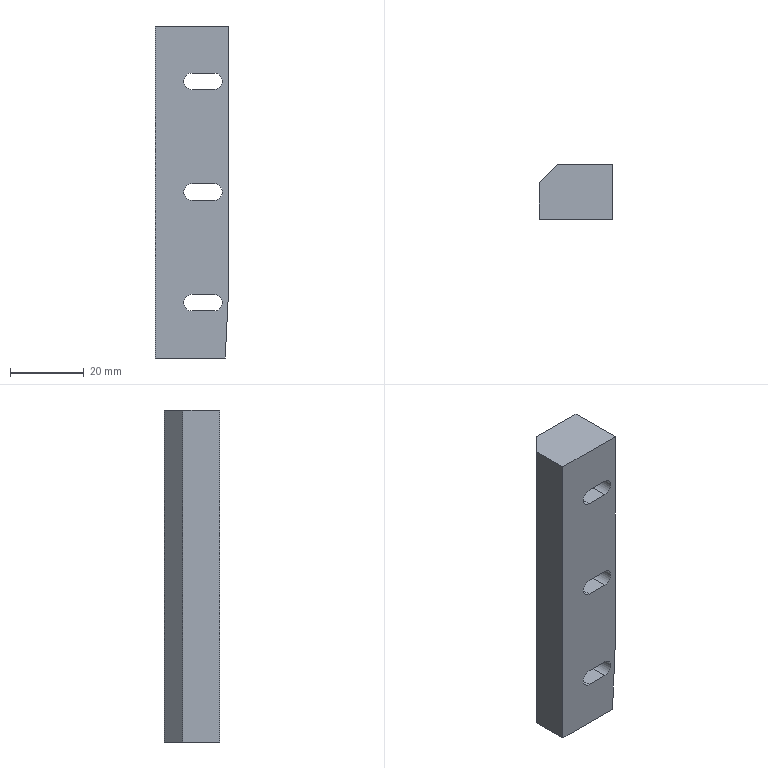Part | SolidWorks | features Cut 3, Chamfer 1, Extrusion 1, LPattern 1 | 1 solid | 36 faces | box 20 x 15 x 90 mm | volume 22961 mm3 | plane 23 | cylinder 13 | commonest cylinder face diameters 7.5 x7 4.5 x6
STEP:
#1=CARTESIAN_POINT('',(0.,9.,32.25));
#2=VERTEX_POINT('',#1);
#3=CARTESIAN_POINT('',(0.,9.,27.75));
#4=VERTEX_POINT('',#3);
#5=CARTESIAN_POINT('',(0.,9.,30.));
#6=DIRECTION('',(0.,-1.,0.));
#7=DIRECTION('',(0.,0.,1.));
#8=AXIS2_PLACEMENT_3D('',#5,#6,#7);
#9=CIRCLE('',#8,2.25);
#10=EDGE_CURVE('',#2,#4,#9,.T.);
#11=ORIENTED_EDGE('',*,*,#10,.F.);
#12=CARTESIAN_POINT('',(0.,0.,32.25));
#13=VERTEX_POINT('',#12);
#14=CARTESIAN_POINT('',(0.,0.,32.25));
#15=DIRECTION('',(0.,1.,0.));
#16=VECTOR('',#15,1000.);
#17=LINE('',#14,#16);
#18=EDGE_CURVE('',#13,#2,#17,.T.);
#19=ORIENTED_EDGE('',*,*,#18,.F.);
#20=CARTESIAN_POINT('',(0.,0.,27.75));
#21=VERTEX_POINT('',#20);
#22=CARTESIAN_POINT('',(0.,0.,30.));
#23=DIRECTION('',(0.,1.,0.));
#24=DIRECTION('',(0.,0.,1.));
#25=AXIS2_PLACEMENT_3D('',#22,#23,#24);
#26=CIRCLE('',#25,2.25);
#27=EDGE_CURVE('',#21,#13,#26,.T.);
#28=ORIENTED_EDGE('',*,*,#27,.F.);
#29=CARTESIAN_POINT('',(0.,0.,27.75));
#30=DIRECTION('',(0.,1.,0.));
#31=VECTOR('',#30,1000.);
#32=LINE('',#29,#31);
#33=EDGE_CURVE('',#21,#4,#32,.T.);
#34=ORIENTED_EDGE('',*,*,#33,.T.);
#35=EDGE_LOOP('',(#11,#19,#28,#34));
#36=FACE_OUTER_BOUND('',#35,.T.);
#37=CARTESIAN_POINT('',(0.,0.,30.));
#38=DIRECTION('',(0.,1.,0.));
#39=DIRECTION('',(0.,0.,1.));
#40=AXIS2_PLACEMENT_3D('',#37,#38,#39);
#41=CYLINDRICAL_SURFACE('',#40,2.25);
#42=ADVANCED_FACE('',(#36),#41,.F.);
#43=CARTESIAN_POINT('',(6.,9.,27.75));
#44=VERTEX_POINT('',#43);
#45=CARTESIAN_POINT('',(0.,9.,27.75));
#46=DIRECTION('',(1.,0.,0.));
#47=VECTOR('',#46,1000.);
#48=LINE('',#45,#47);
#49=EDGE_CURVE('',#4,#44,#48,.T.);
#50=ORIENTED_EDGE('',*,*,#49,.F.);
#51=ORIENTED_EDGE('',*,*,#33,.F.);
#52=CARTESIAN_POINT('',(6.,0.,27.75));
#53=VERTEX_POINT('',#52);
#54=CARTESIAN_POINT('',(0.,0.,27.75));
#55=DIRECTION('',(-1.,0.,0.));
#56=VECTOR('',#55,1000.);
#57=LINE('',#54,#56);
#58=EDGE_CURVE('',#53,#21,#57,.T.);
#59=ORIENTED_EDGE('',*,*,#58,.F.);
#60=CARTESIAN_POINT('',(6.,0.,27.75));
#61=DIRECTION('',(0.,1.,0.));
#62=VECTOR('',#61,1000.);
#63=LINE('',#60,#62);
#64=EDGE_CURVE('',#53,#44,#63,.T.);
#65=ORIENTED_EDGE('',*,*,#64,.T.);
#66=EDGE_LOOP('',(#50,#51,#59,#65));
#67=FACE_OUTER_BOUND('',#66,.T.);
#68=CARTESIAN_POINT('',(0.,0.,27.75));
#69=DIRECTION('',(0.,0.,-1.));
#70=DIRECTION('',(-1.,0.,0.));
#71=AXIS2_PLACEMENT_3D('',#68,#69,#70);
#72=PLANE('',#71);
#73=ADVANCED_FACE('',(#67),#72,.F.);
#74=CARTESIAN_POINT('',(6.,9.,32.25));
#75=VERTEX_POINT('',#74);
#76=CARTESIAN_POINT('',(6.,9.,30.));
#77=DIRECTION('',(0.,-1.,0.));
#78=DIRECTION('',(0.,0.,1.));
#79=AXIS2_PLACEMENT_3D('',#76,#77,#78);
#80=CIRCLE('',#79,2.25);
#81=EDGE_CURVE('',#44,#75,#80,.T.);
#82=ORIENTED_EDGE('',*,*,#81,.F.);
#83=ORIENTED_EDGE('',*,*,#64,.F.);
#84=CARTESIAN_POINT('',(6.,0.,32.25));
#85=VERTEX_POINT('',#84);
#86=CARTESIAN_POINT('',(6.,0.,30.));
#87=DIRECTION('',(0.,1.,0.));
#88=DIRECTION('',(0.,0.,1.));
#89=AXIS2_PLACEMENT_3D('',#86,#87,#88);
#90=CIRCLE('',#89,2.25);
#91=EDGE_CURVE('',#85,#53,#90,.T.);
#92=ORIENTED_EDGE('',*,*,#91,.F.);
#93=CARTESIAN_POINT('',(6.,0.,32.25));
#94=DIRECTION('',(0.,1.,0.));
#95=VECTOR('',#94,1000.);
#96=LINE('',#93,#95);
#97=EDGE_CURVE('',#85,#75,#96,.T.);
#98=ORIENTED_EDGE('',*,*,#97,.T.);
#99=EDGE_LOOP('',(#82,#83,#92,#98));
#100=FACE_OUTER_BOUND('',#99,.T.);
#101=CARTESIAN_POINT('',(6.,0.,30.));
#102=DIRECTION('',(0.,1.,0.));
#103=DIRECTION('',(0.,0.,1.));
#104=AXIS2_PLACEMENT_3D('',#101,#102,#103);
#105=CYLINDRICAL_SURFACE('',#104,2.25);
#106=ADVANCED_FACE('',(#100),#105,.F.);
#107=CARTESIAN_POINT('',(0.,9.,32.25));
#108=DIRECTION('',(-1.,0.,0.));
#109=VECTOR('',#108,1000.);
#110=LINE('',#107,#109);
#111=EDGE_CURVE('',#75,#2,#110,.T.);
#112=ORIENTED_EDGE('',*,*,#111,.F.);
#113=ORIENTED_EDGE('',*,*,#97,.F.);
#114=CARTESIAN_POINT('',(0.,0.,32.25));
#115=DIRECTION('',(1.,0.,0.));
#116=VECTOR('',#115,1000.);
#117=LINE('',#114,#116);
#118=EDGE_CURVE('',#13,#85,#117,.T.);
#119=ORIENTED_EDGE('',*,*,#118,.F.);
#120=ORIENTED_EDGE('',*,*,#18,.T.);
#121=EDGE_LOOP('',(#112,#113,#119,#120));
#122=FACE_OUTER_BOUND('',#121,.T.);
#123=CARTESIAN_POINT('',(0.,0.,32.25));
#124=DIRECTION('',(0.,0.,1.));
#125=DIRECTION('',(1.,0.,0.));
#126=AXIS2_PLACEMENT_3D('',#123,#124,#125);
#127=PLANE('',#126);
#128=ADVANCED_FACE('',(#122),#127,.F.);
#129=CARTESIAN_POINT('',(0.,9.,-27.75));
#130=VERTEX_POINT('',#129);
#131=CARTESIAN_POINT('',(0.,9.,-32.25));
#132=VERTEX_POINT('',#131);
#133=CARTESIAN_POINT('',(0.,9.,-30.));
#134=DIRECTION('',(0.,-1.,0.));
#135=DIRECTION('',(0.,0.,1.));
#136=AXIS2_PLACEMENT_3D('',#133,#134,#135);
#137=CIRCLE('',#136,2.25);
#138=EDGE_CURVE('',#130,#132,#137,.T.);
#139=ORIENTED_EDGE('',*,*,#138,.F.);
#140=CARTESIAN_POINT('',(0.,0.,-27.75));
#141=VERTEX_POINT('',#140);
#142=CARTESIAN_POINT('',(0.,0.,-27.75));
#143=DIRECTION('',(0.,1.,0.));
#144=VECTOR('',#143,1000.);
#145=LINE('',#142,#144);
#146=EDGE_CURVE('',#141,#130,#145,.T.);
#147=ORIENTED_EDGE('',*,*,#146,.F.);
#148=CARTESIAN_POINT('',(0.,0.,-32.25));
#149=VERTEX_POINT('',#148);
#150=CARTESIAN_POINT('',(0.,0.,-30.));
#151=DIRECTION('',(0.,1.,0.));
#152=DIRECTION('',(0.,0.,1.));
#153=AXIS2_PLACEMENT_3D('',#150,#151,#152);
#154=CIRCLE('',#153,2.25);
#155=EDGE_CURVE('',#149,#141,#154,.T.);
#156=ORIENTED_EDGE('',*,*,#155,.F.);
#157=CARTESIAN_POINT('',(0.,0.,-32.25));
#158=DIRECTION('',(0.,1.,0.));
#159=VECTOR('',#158,1000.);
#160=LINE('',#157,#159);
#161=EDGE_CURVE('',#149,#132,#160,.T.);
#162=ORIENTED_EDGE('',*,*,#161,.T.);
#163=EDGE_LOOP('',(#139,#147,#156,#162));
#164=FACE_OUTER_BOUND('',#163,.T.);
#165=CARTESIAN_POINT('',(0.,0.,-30.));
#166=DIRECTION('',(0.,1.,0.));
#167=DIRECTION('',(0.,0.,1.));
#168=AXIS2_PLACEMENT_3D('',#165,#166,#167);
#169=CYLINDRICAL_SURFACE('',#168,2.25);
#170=ADVANCED_FACE('',(#164),#169,.F.);
#171=CARTESIAN_POINT('',(6.,9.,-32.25));
#172=VERTEX_POINT('',#171);
#173=CARTESIAN_POINT('',(0.,9.,-32.25));
#174=DIRECTION('',(1.,0.,0.));
#175=VECTOR('',#174,1000.);
#176=LINE('',#173,#175);
#177=EDGE_CURVE('',#132,#172,#176,.T.);
#178=ORIENTED_EDGE('',*,*,#177,.F.);
#179=ORIENTED_EDGE('',*,*,#161,.F.);
#180=CARTESIAN_POINT('',(6.,0.,-32.25));
#181=VERTEX_POINT('',#180);
#182=CARTESIAN_POINT('',(0.,0.,-32.25));
#183=DIRECTION('',(-1.,0.,0.));
#184=VECTOR('',#183,1000.);
#185=LINE('',#182,#184);
#186=EDGE_CURVE('',#181,#149,#185,.T.);
#187=ORIENTED_EDGE('',*,*,#186,.F.);
#188=CARTESIAN_POINT('',(6.,0.,-32.25));
#189=DIRECTION('',(0.,1.,0.));
#190=VECTOR('',#189,1000.);
#191=LINE('',#188,#190);
#192=EDGE_CURVE('',#181,#172,#191,.T.);
#193=ORIENTED_EDGE('',*,*,#192,.T.);
#194=EDGE_LOOP('',(#178,#179,#187,#193));
#195=FACE_OUTER_BOUND('',#194,.T.);
#196=CARTESIAN_POINT('',(0.,0.,-32.25));
#197=DIRECTION('',(0.,0.,-1.));
#198=DIRECTION('',(-1.,0.,0.));
#199=AXIS2_PLACEMENT_3D('',#196,#197,#198);
#200=PLANE('',#199);
#201=ADVANCED_FACE('',(#195),#200,.F.);
#202=CARTESIAN_POINT('',(6.,9.,-27.75));
#203=VERTEX_POINT('',#202);
#204=CARTESIAN_POINT('',(6.,9.,-30.));
#205=DIRECTION('',(0.,-1.,0.));
#206=DIRECTION('',(0.,0.,1.));
#207=AXIS2_PLACEMENT_3D('',#204,#205,#206);
#208=CIRCLE('',#207,2.25);
#209=EDGE_CURVE('',#172,#203,#208,.T.);
#210=ORIENTED_EDGE('',*,*,#209,.F.);
#211=ORIENTED_EDGE('',*,*,#192,.F.);
#212=CARTESIAN_POINT('',(6.,0.,-27.75));
#213=VERTEX_POINT('',#212);
#214=CARTESIAN_POINT('',(6.,0.,-30.));
#215=DIRECTION('',(0.,1.,0.));
#216=DIRECTION('',(0.,0.,1.));
#217=AXIS2_PLACEMENT_3D('',#214,#215,#216);
#218=CIRCLE('',#217,2.25);
#219=EDGE_CURVE('',#213,#181,#218,.T.);
#220=ORIENTED_EDGE('',*,*,#219,.F.);
#221=CARTESIAN_POINT('',(6.,0.,-27.75));
#222=DIRECTION('',(0.,1.,0.));
#223=VECTOR('',#222,1000.);
#224=LINE('',#221,#223);
#225=EDGE_CURVE('',#213,#203,#224,.T.);
#226=ORIENTED_EDGE('',*,*,#225,.T.);
#227=EDGE_LOOP('',(#210,#211,#220,#226));
#228=FACE_OUTER_BOUND('',#227,.T.);
#229=CARTESIAN_POINT('',(6.,0.,-30.));
#230=DIRECTION('',(0.,1.,0.));
#231=DIRECTION('',(0.,0.,1.));
#232=AXIS2_PLACEMENT_3D('',#229,#230,#231);
#233=CYLINDRICAL_SURFACE('',#232,2.25);
#234=ADVANCED_FACE('',(#228),#233,.F.);
#235=CARTESIAN_POINT('',(0.,9.,-27.75));
#236=DIRECTION('',(-1.,0.,0.));
#237=VECTOR('',#236,1000.);
#238=LINE('',#235,#237);
#239=EDGE_CURVE('',#203,#130,#238,.T.);
#240=ORIENTED_EDGE('',*,*,#239,.F.);
#241=ORIENTED_EDGE('',*,*,#225,.F.);
#242=CARTESIAN_POINT('',(0.,0.,-27.75));
#243=DIRECTION('',(1.,0.,0.));
#244=VECTOR('',#243,1000.);
#245=LINE('',#242,#244);
#246=EDGE_CURVE('',#141,#213,#245,.T.);
#247=ORIENTED_EDGE('',*,*,#246,.F.);
#248=ORIENTED_EDGE('',*,*,#146,.T.);
#249=EDGE_LOOP('',(#240,#241,#247,#248));
#250=FACE_OUTER_BOUND('',#249,.T.);
#251=CARTESIAN_POINT('',(0.,0.,-27.75));
#252=DIRECTION('',(0.,0.,1.));
#253=DIRECTION('',(1.,0.,0.));
#254=AXIS2_PLACEMENT_3D('',#251,#252,#253);
#255=PLANE('',#254);
#256=ADVANCED_FACE('',(#250),#255,.F.);
#257=CARTESIAN_POINT('',(0.,9.,2.25));
#258=VERTEX_POINT('',#257);
#259=CARTESIAN_POINT('',(0.,9.,-2.25));
#260=VERTEX_POINT('',#259);
#261=CARTESIAN_POINT('',(0.,9.,0.));
#262=DIRECTION('',(0.,-1.,0.));
#263=DIRECTION('',(0.,0.,1.));
#264=AXIS2_PLACEMENT_3D('',#261,#262,#263);
#265=CIRCLE('',#264,2.25);
#266=EDGE_CURVE('',#258,#260,#265,.T.);
#267=ORIENTED_EDGE('',*,*,#266,.F.);
#268=CARTESIAN_POINT('',(0.,0.,2.25));
#269=VERTEX_POINT('',#268);
#270=CARTESIAN_POINT('',(0.,0.,2.25));
#271=DIRECTION('',(0.,1.,0.));
#272=VECTOR('',#271,1000.);
#273=LINE('',#270,#272);
#274=EDGE_CURVE('',#269,#258,#273,.T.);
#275=ORIENTED_EDGE('',*,*,#274,.F.);
#276=CARTESIAN_POINT('',(0.,0.,-2.25));
#277=VERTEX_POINT('',#276);
#278=CARTESIAN_POINT('',(0.,0.,0.));
#279=DIRECTION('',(0.,1.,0.));
#280=DIRECTION('',(0.,0.,1.));
#281=AXIS2_PLACEMENT_3D('',#278,#279,#280);
#282=CIRCLE('',#281,2.25);
#283=EDGE_CURVE('',#277,#269,#282,.T.);
#284=ORIENTED_EDGE('',*,*,#283,.F.);
#285=CARTESIAN_POINT('',(0.,0.,-2.25));
#286=DIRECTION('',(0.,1.,0.));
#287=VECTOR('',#286,1000.);
#288=LINE('',#285,#287);
#289=EDGE_CURVE('',#277,#260,#288,.T.);
#290=ORIENTED_EDGE('',*,*,#289,.T.);
#291=EDGE_LOOP('',(#267,#275,#284,#290));
#292=FACE_OUTER_BOUND('',#291,.T.);
#293=CARTESIAN_POINT('',(0.,0.,0.));
#294=DIRECTION('',(0.,1.,0.));
#295=DIRECTION('',(0.,0.,1.));
#296=AXIS2_PLACEMENT_3D('',#293,#294,#295);
#297=CYLINDRICAL_SURFACE('',#296,2.25);
#298=ADVANCED_FACE('',(#292),#297,.F.);
#299=CARTESIAN_POINT('',(6.,9.,-2.25));
#300=VERTEX_POINT('',#299);
#301=CARTESIAN_POINT('',(0.,9.,-2.25));
#302=DIRECTION('',(1.,0.,0.));
#303=VECTOR('',#302,1000.);
#304=LINE('',#301,#303);
#305=EDGE_CURVE('',#260,#300,#304,.T.);
#306=ORIENTED_EDGE('',*,*,#305,.F.);
#307=ORIENTED_EDGE('',*,*,#289,.F.);
#308=CARTESIAN_POINT('',(6.,0.,-2.25));
#309=VERTEX_POINT('',#308);
#310=CARTESIAN_POINT('',(0.,0.,-2.25));
#311=DIRECTION('',(-1.,0.,0.));
#312=VECTOR('',#311,1000.);
#313=LINE('',#310,#312);
#314=EDGE_CURVE('',#309,#277,#313,.T.);
#315=ORIENTED_EDGE('',*,*,#314,.F.);
#316=CARTESIAN_POINT('',(6.,0.,-2.25));
#317=DIRECTION('',(0.,1.,0.));
#318=VECTOR('',#317,1000.);
#319=LINE('',#316,#318);
#320=EDGE_CURVE('',#309,#300,#319,.T.);
#321=ORIENTED_EDGE('',*,*,#320,.T.);
#322=EDGE_LOOP('',(#306,#307,#315,#321));
#323=FACE_OUTER_BOUND('',#322,.T.);
#324=CARTESIAN_POINT('',(0.,0.,-2.25));
#325=DIRECTION('',(0.,0.,-1.));
#326=DIRECTION('',(-1.,0.,0.));
#327=AXIS2_PLACEMENT_3D('',#324,#325,#326);
#328=PLANE('',#327);
#329=ADVANCED_FACE('',(#323),#328,.F.);
#330=CARTESIAN_POINT('',(6.,9.,2.25));
#331=VERTEX_POINT('',#330);
#332=CARTESIAN_POINT('',(6.,9.,0.));
#333=DIRECTION('',(0.,-1.,0.));
#334=DIRECTION('',(0.,0.,1.));
#335=AXIS2_PLACEMENT_3D('',#332,#333,#334);
#336=CIRCLE('',#335,2.25);
#337=EDGE_CURVE('',#300,#331,#336,.T.);
#338=ORIENTED_EDGE('',*,*,#337,.F.);
#339=ORIENTED_EDGE('',*,*,#320,.F.);
#340=CARTESIAN_POINT('',(6.,0.,2.25));
#341=VERTEX_POINT('',#340);
#342=CARTESIAN_POINT('',(6.,0.,0.));
#343=DIRECTION('',(0.,1.,0.));
#344=DIRECTION('',(0.,0.,1.));
#345=AXIS2_PLACEMENT_3D('',#342,#343,#344);
#346=CIRCLE('',#345,2.25);
#347=EDGE_CURVE('',#341,#309,#346,.T.);
#348=ORIENTED_EDGE('',*,*,#347,.F.);
#349=CARTESIAN_POINT('',(6.,0.,2.25));
#350=DIRECTION('',(0.,1.,0.));
#351=VECTOR('',#350,1000.);
#352=LINE('',#349,#351);
#353=EDGE_CURVE('',#341,#331,#352,.T.);
#354=ORIENTED_EDGE('',*,*,#353,.T.);
#355=EDGE_LOOP('',(#338,#339,#348,#354));
#356=FACE_OUTER_BOUND('',#355,.T.);
#357=CARTESIAN_POINT('',(6.,0.,0.));
#358=DIRECTION('',(0.,1.,0.));
#359=DIRECTION('',(0.,0.,1.));
#360=AXIS2_PLACEMENT_3D('',#357,#358,#359);
#361=CYLINDRICAL_SURFACE('',#360,2.25);
#362=ADVANCED_FACE('',(#356),#361,.F.);
#363=CARTESIAN_POINT('',(0.,9.,2.25));
#364=DIRECTION('',(-1.,0.,0.));
#365=VECTOR('',#364,1000.);
#366=LINE('',#363,#365);
#367=EDGE_CURVE('',#331,#258,#366,.T.);
#368=ORIENTED_EDGE('',*,*,#367,.F.);
#369=ORIENTED_EDGE('',*,*,#353,.F.);
#370=CARTESIAN_POINT('',(0.,0.,2.25));
#371=DIRECTION('',(1.,0.,0.));
#372=VECTOR('',#371,1000.);
#373=LINE('',#370,#372);
#374=EDGE_CURVE('',#269,#341,#373,.T.);
#375=ORIENTED_EDGE('',*,*,#374,.F.);
#376=ORIENTED_EDGE('',*,*,#274,.T.);
#377=EDGE_LOOP('',(#368,#369,#375,#376));
#378=FACE_OUTER_BOUND('',#377,.T.);
#379=CARTESIAN_POINT('',(0.,0.,2.25));
#380=DIRECTION('',(0.,0.,1.));
#381=DIRECTION('',(1.,0.,0.));
#382=AXIS2_PLACEMENT_3D('',#379,#380,#381);
#383=PLANE('',#382);
#384=ADVANCED_FACE('',(#378),#383,.F.);
#385=CARTESIAN_POINT('',(10.,0.,45.));
#386=VERTEX_POINT('',#385);
#387=CARTESIAN_POINT('',(10.,0.,-25.));
#388=VERTEX_POINT('',#387);
#389=CARTESIAN_POINT('',(10.,0.,-45.));
#390=DIRECTION('',(0.,0.,-1.));
#391=VECTOR('',#390,1000.);
#392=LINE('',#389,#391);
#393=EDGE_CURVE('',#386,#388,#392,.T.);
#394=ORIENTED_EDGE('',*,*,#393,.T.);
#395=CARTESIAN_POINT('',(10.,15.,-25.));
#396=VERTEX_POINT('',#395);
#397=CARTESIAN_POINT('',(10.,0.,-25.));
#398=DIRECTION('',(0.,1.,0.));
#399=VECTOR('',#398,1000.);
#400=LINE('',#397,#399);
#401=EDGE_CURVE('',#388,#396,#400,.T.);
#402=ORIENTED_EDGE('',*,*,#401,.T.);
#403=CARTESIAN_POINT('',(10.,15.,45.));
#404=VERTEX_POINT('',#403);
#405=CARTESIAN_POINT('',(10.,15.,-45.));
#406=DIRECTION('',(0.,0.,-1.));
#407=VECTOR('',#406,1000.);
#408=LINE('',#405,#407);
#409=EDGE_CURVE('',#404,#396,#408,.T.);
#410=ORIENTED_EDGE('',*,*,#409,.F.);
#411=CARTESIAN_POINT('',(10.,15.,45.));
#412=DIRECTION('',(0.,-1.,0.));
#413=VECTOR('',#412,1000.);
#414=LINE('',#411,#413);
#415=EDGE_CURVE('',#404,#386,#414,.T.);
#416=ORIENTED_EDGE('',*,*,#415,.T.);
#417=EDGE_LOOP('',(#394,#402,#410,#416));
#418=FACE_OUTER_BOUND('',#417,.T.);
#419=CARTESIAN_POINT('',(10.,15.,-45.));
#420=DIRECTION('',(-1.,0.,0.));
#421=DIRECTION('',(0.,0.,1.));
#422=AXIS2_PLACEMENT_3D('',#419,#420,#421);
#423=PLANE('',#422);
#424=ADVANCED_FACE('',(#418),#423,.F.);
#425=CARTESIAN_POINT('',(9.,15.,-45.));
#426=VERTEX_POINT('',#425);
#427=CARTESIAN_POINT('',(-5.,15.,-45.));
#428=VERTEX_POINT('',#427);
#429=CARTESIAN_POINT('',(-10.,15.,-45.));
#430=DIRECTION('',(-1.,0.,0.));
#431=VECTOR('',#430,1000.);
#432=LINE('',#429,#431);
#433=EDGE_CURVE('',#426,#428,#432,.T.);
#434=ORIENTED_EDGE('',*,*,#433,.F.);
#435=CARTESIAN_POINT('',(9.,0.,-45.));
#436=VERTEX_POINT('',#435);
#437=CARTESIAN_POINT('',(9.,0.,-45.));
#438=DIRECTION('',(0.,1.,0.));
#439=VECTOR('',#438,1000.);
#440=LINE('',#437,#439);
#441=EDGE_CURVE('',#436,#426,#440,.T.);
#442=ORIENTED_EDGE('',*,*,#441,.F.);
#443=CARTESIAN_POINT('',(-10.,0.,-45.));
#444=VERTEX_POINT('',#443);
#445=CARTESIAN_POINT('',(-10.,0.,-45.));
#446=DIRECTION('',(-1.,0.,0.));
#447=VECTOR('',#446,1000.);
#448=LINE('',#445,#447);
#449=EDGE_CURVE('',#436,#444,#448,.T.);
#450=ORIENTED_EDGE('',*,*,#449,.T.);
#451=CARTESIAN_POINT('',(-10.,10.,-45.));
#452=VERTEX_POINT('',#451);
#453=CARTESIAN_POINT('',(-10.,15.,-45.));
#454=DIRECTION('',(0.,-1.,0.));
#455=VECTOR('',#454,1000.);
#456=LINE('',#453,#455);
#457=EDGE_CURVE('',#452,#444,#456,.T.);
#458=ORIENTED_EDGE('',*,*,#457,.F.);
#459=CARTESIAN_POINT('',(-5.,15.,-45.));
#460=DIRECTION('',(0.7071,0.7071,0.));
#461=VECTOR('',#460,1000.);
#462=LINE('',#459,#461);
#463=EDGE_CURVE('',#452,#428,#462,.T.);
#464=ORIENTED_EDGE('',*,*,#463,.T.);
#465=EDGE_LOOP('',(#434,#442,#450,#458,#464));
#466=FACE_OUTER_BOUND('',#465,.T.);
#467=CARTESIAN_POINT('',(-10.,15.,-45.));
#468=DIRECTION('',(0.,0.,1.));
#469=DIRECTION('',(1.,0.,0.));
#470=AXIS2_PLACEMENT_3D('',#467,#468,#469);
#471=PLANE('',#470);
#472=ADVANCED_FACE('',(#466),#471,.F.);
#473=CARTESIAN_POINT('',(-10.,10.,45.));
#474=VERTEX_POINT('',#473);
#475=CARTESIAN_POINT('',(-10.,0.,45.));
#476=VERTEX_POINT('',#475);
#477=CARTESIAN_POINT('',(-10.,15.,45.));
#478=DIRECTION('',(0.,-1.,0.));
#479=VECTOR('',#478,1000.);
#480=LINE('',#477,#479);
#481=EDGE_CURVE('',#474,#476,#480,.T.);
#482=ORIENTED_EDGE('',*,*,#481,.F.);
#483=CARTESIAN_POINT('',(-10.,10.,-45.));
#484=DIRECTION('',(0.,0.,-1.));
#485=VECTOR('',#484,1000.);
#486=LINE('',#483,#485);
#487=EDGE_CURVE('',#474,#452,#486,.T.);
#488=ORIENTED_EDGE('',*,*,#487,.T.);
#489=ORIENTED_EDGE('',*,*,#457,.T.);
#490=CARTESIAN_POINT('',(-10.,0.,-45.));
#491=DIRECTION('',(0.,0.,1.));
#492=VECTOR('',#491,1000.);
#493=LINE('',#490,#492);
#494=EDGE_CURVE('',#444,#476,#493,.T.);
#495=ORIENTED_EDGE('',*,*,#494,.T.);
#496=EDGE_LOOP('',(#482,#488,#489,#495));
#497=FACE_OUTER_BOUND('',#496,.T.);
#498=CARTESIAN_POINT('',(-10.,15.,-45.));
#499=DIRECTION('',(1.,0.,0.));
#500=DIRECTION('',(0.,0.,-1.));
#501=AXIS2_PLACEMENT_3D('',#498,#499,#500);
#502=PLANE('',#501);
#503=ADVANCED_FACE('',(#497),#502,.F.);
#504=CARTESIAN_POINT('',(-5.,15.,45.));
#505=VERTEX_POINT('',#504);
#506=CARTESIAN_POINT('',(-10.,15.,45.));
#507=DIRECTION('',(1.,0.,0.));
#508=VECTOR('',#507,1000.);
#509=LINE('',#506,#508);
#510=EDGE_CURVE('',#505,#404,#509,.T.);
#511=ORIENTED_EDGE('',*,*,#510,.F.);
#512=CARTESIAN_POINT('',(-5.,15.,45.));
#513=DIRECTION('',(-0.7071,-0.7071,0.));
#514=VECTOR('',#513,1000.);
#515=LINE('',#512,#514);
#516=EDGE_CURVE('',#505,#474,#515,.T.);
#517=ORIENTED_EDGE('',*,*,#516,.T.);
#518=ORIENTED_EDGE('',*,*,#481,.T.);
#519=CARTESIAN_POINT('',(-10.,0.,45.));
#520=DIRECTION('',(1.,0.,0.));
#521=VECTOR('',#520,1000.);
#522=LINE('',#519,#521);
#523=EDGE_CURVE('',#476,#386,#522,.T.);
#524=ORIENTED_EDGE('',*,*,#523,.T.);
#525=ORIENTED_EDGE('',*,*,#415,.F.);
#526=EDGE_LOOP('',(#511,#517,#518,#524,#525));
#527=FACE_OUTER_BOUND('',#526,.T.);
#528=CARTESIAN_POINT('',(-10.,15.,45.));
#529=DIRECTION('',(0.,0.,-1.));
#530=DIRECTION('',(-1.,0.,0.));
#531=AXIS2_PLACEMENT_3D('',#528,#529,#530);
#532=PLANE('',#531);
#533=ADVANCED_FACE('',(#527),#532,.F.);
#534=CARTESIAN_POINT('',(0.,15.,26.25));
#535=VERTEX_POINT('',#534);
#536=CARTESIAN_POINT('',(0.,15.,33.75));
#537=VERTEX_POINT('',#536);
#538=CARTESIAN_POINT('',(0.,15.,30.));
#539=DIRECTION('',(0.,1.,0.));
#540=DIRECTION('',(0.,0.,1.));
#541=AXIS2_PLACEMENT_3D('',#538,#539,#540);
#542=CIRCLE('',#541,3.75);
#543=EDGE_CURVE('',#535,#537,#542,.T.);
#544=ORIENTED_EDGE('',*,*,#543,.F.);
#545=CARTESIAN_POINT('',(6.,15.,26.25));
#546=VERTEX_POINT('',#545);
#547=CARTESIAN_POINT('',(6.,15.,26.25));
#548=DIRECTION('',(-1.,0.,0.));
#549=VECTOR('',#548,1000.);
#550=LINE('',#547,#549);
#551=EDGE_CURVE('',#546,#535,#550,.T.);
#552=ORIENTED_EDGE('',*,*,#551,.F.);
#553=CARTESIAN_POINT('',(6.,15.,33.75));
#554=VERTEX_POINT('',#553);
#555=CARTESIAN_POINT('',(6.,15.,30.));
#556=DIRECTION('',(0.,1.,0.));
#557=DIRECTION('',(0.,0.,1.));
#558=AXIS2_PLACEMENT_3D('',#555,#556,#557);
#559=CIRCLE('',#558,3.75);
#560=EDGE_CURVE('',#554,#546,#559,.T.);
#561=ORIENTED_EDGE('',*,*,#560,.F.);
#562=CARTESIAN_POINT('',(0.,15.,33.75));
#563=DIRECTION('',(1.,0.,0.));
#564=VECTOR('',#563,1000.);
#565=LINE('',#562,#564);
#566=EDGE_CURVE('',#537,#554,#565,.T.);
#567=ORIENTED_EDGE('',*,*,#566,.F.);
#568=EDGE_LOOP('',(#544,#552,#561,#567));
#569=FACE_BOUND('',#568,.T.);
#570=CARTESIAN_POINT('',(9.731,15.,-30.374));
#571=VERTEX_POINT('',#570);
#572=CARTESIAN_POINT('',(6.,15.,-33.75));
#573=VERTEX_POINT('',#572);
#574=CARTESIAN_POINT('',(6.,15.,-30.));
#575=DIRECTION('',(0.,1.,0.));
#576=DIRECTION('',(0.,0.,1.));
#577=AXIS2_PLACEMENT_3D('',#574,#575,#576);
#578=CIRCLE('',#577,3.75);
#579=EDGE_CURVE('',#571,#573,#578,.T.);
#580=ORIENTED_EDGE('',*,*,#579,.F.);
#581=CARTESIAN_POINT('',(10.,15.,-25.));
#582=DIRECTION('',(0.04994,0.,0.9988));
#583=VECTOR('',#582,1000.);
#584=LINE('',#581,#583);
#585=EDGE_CURVE('',#426,#571,#584,.T.);
#586=ORIENTED_EDGE('',*,*,#585,.F.);
#587=ORIENTED_EDGE('',*,*,#433,.T.);
#588=CARTESIAN_POINT('',(-5.,15.,45.));
#589=DIRECTION('',(0.,0.,1.));
#590=VECTOR('',#589,1000.);
#591=LINE('',#588,#590);
#592=EDGE_CURVE('',#428,#505,#591,.T.);
#593=ORIENTED_EDGE('',*,*,#592,.T.);
#594=ORIENTED_EDGE('',*,*,#510,.T.);
#595=ORIENTED_EDGE('',*,*,#409,.T.);
#596=CARTESIAN_POINT('',(9.75,15.,-30.));
#597=VERTEX_POINT('',#596);
#598=CARTESIAN_POINT('',(10.,15.,-25.));
#599=DIRECTION('',(0.04994,0.,0.9988));
#600=VECTOR('',#599,1000.);
#601=LINE('',#598,#600);
#602=EDGE_CURVE('',#597,#396,#601,.T.);
#603=ORIENTED_EDGE('',*,*,#602,.F.);
#604=CARTESIAN_POINT('',(6.,15.,-26.25));
#605=VERTEX_POINT('',#604);
#606=CARTESIAN_POINT('',(6.,15.,-30.));
#607=DIRECTION('',(0.,1.,0.));
#608=DIRECTION('',(0.,0.,1.));
#609=AXIS2_PLACEMENT_3D('',#606,#607,#608);
#610=CIRCLE('',#609,3.75);
#611=EDGE_CURVE('',#605,#597,#610,.T.);
#612=ORIENTED_EDGE('',*,*,#611,.F.);
#613=CARTESIAN_POINT('',(0.,15.,-26.25));
#614=VERTEX_POINT('',#613);
#615=CARTESIAN_POINT('',(0.,15.,-26.25));
#616=DIRECTION('',(1.,0.,0.));
#617=VECTOR('',#616,1000.);
#618=LINE('',#615,#617);
#619=EDGE_CURVE('',#614,#605,#618,.T.);
#620=ORIENTED_EDGE('',*,*,#619,.F.);
#621=CARTESIAN_POINT('',(0.,15.,-33.75));
#622=VERTEX_POINT('',#621);
#623=CARTESIAN_POINT('',(0.,15.,-30.));
#624=DIRECTION('',(0.,1.,0.));
#625=DIRECTION('',(0.,0.,1.));
#626=AXIS2_PLACEMENT_3D('',#623,#624,#625);
#627=CIRCLE('',#626,3.75);
#628=EDGE_CURVE('',#622,#614,#627,.T.);
#629=ORIENTED_EDGE('',*,*,#628,.F.);
#630=CARTESIAN_POINT('',(6.,15.,-33.75));
#631=DIRECTION('',(-1.,0.,0.));
#632=VECTOR('',#631,1000.);
#633=LINE('',#630,#632);
#634=EDGE_CURVE('',#573,#622,#633,.T.);
#635=ORIENTED_EDGE('',*,*,#634,.F.);
#636=EDGE_LOOP('',(#580,#586,#587,#593,#594,#595,#603,#612,#620,#629,#635));
#637=FACE_OUTER_BOUND('',#636,.T.);
#638=CARTESIAN_POINT('',(0.,15.,-3.75));
#639=VERTEX_POINT('',#638);
#640=CARTESIAN_POINT('',(0.,15.,3.75));
#641=VERTEX_POINT('',#640);
#642=CARTESIAN_POINT('',(0.,15.,0.));
#643=DIRECTION('',(0.,1.,0.));
#644=DIRECTION('',(0.,0.,1.));
#645=AXIS2_PLACEMENT_3D('',#642,#643,#644);
#646=CIRCLE('',#645,3.75);
#647=EDGE_CURVE('',#639,#641,#646,.T.);
#648=ORIENTED_EDGE('',*,*,#647,.F.);
#649=CARTESIAN_POINT('',(6.,15.,-3.75));
#650=VERTEX_POINT('',#649);
#651=CARTESIAN_POINT('',(6.,15.,-3.75));
#652=DIRECTION('',(-1.,0.,0.));
#653=VECTOR('',#652,1000.);
#654=LINE('',#651,#653);
#655=EDGE_CURVE('',#650,#639,#654,.T.);
#656=ORIENTED_EDGE('',*,*,#655,.F.);
#657=CARTESIAN_POINT('',(6.,15.,3.75));
#658=VERTEX_POINT('',#657);
#659=CARTESIAN_POINT('',(6.,15.,0.));
#660=DIRECTION('',(0.,1.,0.));
#661=DIRECTION('',(0.,0.,1.));
#662=AXIS2_PLACEMENT_3D('',#659,#660,#661);
#663=CIRCLE('',#662,3.75);
#664=EDGE_CURVE('',#658,#650,#663,.T.);
#665=ORIENTED_EDGE('',*,*,#664,.F.);
#666=CARTESIAN_POINT('',(0.,15.,3.75));
#667=DIRECTION('',(1.,0.,0.));
#668=VECTOR('',#667,1000.);
#669=LINE('',#666,#668);
#670=EDGE_CURVE('',#641,#658,#669,.T.);
#671=ORIENTED_EDGE('',*,*,#670,.F.);
#672=EDGE_LOOP('',(#648,#656,#665,#671));
#673=FACE_BOUND('',#672,.T.);
#674=CARTESIAN_POINT('',(0.,15.,0.));
#675=DIRECTION('',(0.,1.,0.));
#676=DIRECTION('',(0.,0.,1.));
#677=AXIS2_PLACEMENT_3D('',#674,#675,#676);
#678=PLANE('',#677);
#679=ADVANCED_FACE('',(#569,#637,#673),#678,.T.);
#680=ORIENTED_EDGE('',*,*,#58,.T.);
#681=ORIENTED_EDGE('',*,*,#27,.T.);
#682=ORIENTED_EDGE('',*,*,#118,.T.);
#683=ORIENTED_EDGE('',*,*,#91,.T.);
#684=EDGE_LOOP('',(#680,#681,#682,#683));
#685=FACE_BOUND('',#684,.T.);
#686=ORIENTED_EDGE('',*,*,#186,.T.);
#687=ORIENTED_EDGE('',*,*,#155,.T.);
#688=ORIENTED_EDGE('',*,*,#246,.T.);
#689=ORIENTED_EDGE('',*,*,#219,.T.);
#690=EDGE_LOOP('',(#686,#687,#688,#689));
#691=FACE_BOUND('',#690,.T.);
#692=ORIENTED_EDGE('',*,*,#314,.T.);
#693=ORIENTED_EDGE('',*,*,#283,.T.);
#694=ORIENTED_EDGE('',*,*,#374,.T.);
#695=ORIENTED_EDGE('',*,*,#347,.T.);
#696=EDGE_LOOP('',(#692,#693,#694,#695));
#697=FACE_BOUND('',#696,.T.);
#698=ORIENTED_EDGE('',*,*,#449,.F.);
#699=CARTESIAN_POINT('',(10.,0.,-25.));
#700=DIRECTION('',(0.04994,0.,0.9988));
#701=VECTOR('',#700,1000.);
#702=LINE('',#699,#701);
#703=EDGE_CURVE('',#436,#388,#702,.T.);
#704=ORIENTED_EDGE('',*,*,#703,.T.);
#705=ORIENTED_EDGE('',*,*,#393,.F.);
#706=ORIENTED_EDGE('',*,*,#523,.F.);
#707=ORIENTED_EDGE('',*,*,#494,.F.);
#708=EDGE_LOOP('',(#698,#704,#705,#706,#707));
#709=FACE_OUTER_BOUND('',#708,.T.);
#710=CARTESIAN_POINT('',(0.,0.,0.));
#711=DIRECTION('',(0.,1.,0.));
#712=DIRECTION('',(0.,0.,1.));
#713=AXIS2_PLACEMENT_3D('',#710,#711,#712);
#714=PLANE('',#713);
#715=ADVANCED_FACE('',(#685,#691,#697,#709),#714,.F.);
#716=ORIENTED_EDGE('',*,*,#463,.F.);
#717=ORIENTED_EDGE('',*,*,#487,.F.);
#718=ORIENTED_EDGE('',*,*,#516,.F.);
#719=ORIENTED_EDGE('',*,*,#592,.F.);
#720=EDGE_LOOP('',(#716,#717,#718,#719));
#721=FACE_OUTER_BOUND('',#720,.T.);
#722=CARTESIAN_POINT('',(-5.,15.,0.));
#723=DIRECTION('',(-0.7071,0.7071,0.));
#724=DIRECTION('',(0.,0.,-1.));
#725=AXIS2_PLACEMENT_3D('',#722,#723,#724);
#726=PLANE('',#725);
#727=ADVANCED_FACE('',(#721),#726,.T.);
#728=CARTESIAN_POINT('',(9.75,9.,-30.));
#729=VERTEX_POINT('',#728);
#730=CARTESIAN_POINT('',(9.731,9.,-30.374));
#731=VERTEX_POINT('',#730);
#732=CARTESIAN_POINT('',(9.75,9.,-30.));
#733=DIRECTION('',(-0.04994,0.,-0.9988));
#734=VECTOR('',#733,1000.);
#735=LINE('',#732,#734);
#736=EDGE_CURVE('',#729,#731,#735,.T.);
#737=ORIENTED_EDGE('',*,*,#736,.F.);
#738=CARTESIAN_POINT('',(9.75,9.,-30.));
#739=DIRECTION('',(0.,1.,0.));
#740=VECTOR('',#739,1000.);
#741=LINE('',#738,#740);
#742=EDGE_CURVE('',#729,#597,#741,.T.);
#743=ORIENTED_EDGE('',*,*,#742,.T.);
#744=ORIENTED_EDGE('',*,*,#602,.T.);
#745=ORIENTED_EDGE('',*,*,#401,.F.);
#746=ORIENTED_EDGE('',*,*,#703,.F.);
#747=ORIENTED_EDGE('',*,*,#441,.T.);
#748=ORIENTED_EDGE('',*,*,#585,.T.);
#749=CARTESIAN_POINT('',(9.731,9.,-30.374));
#750=DIRECTION('',(0.,-1.,0.));
#751=VECTOR('',#750,1000.);
#752=LINE('',#749,#751);
#753=EDGE_CURVE('',#571,#731,#752,.T.);
#754=ORIENTED_EDGE('',*,*,#753,.T.);
#755=EDGE_LOOP('',(#737,#743,#744,#745,#746,#747,#748,#754));
#756=FACE_OUTER_BOUND('',#755,.T.);
#757=CARTESIAN_POINT('',(10.,0.,-25.));
#758=DIRECTION('',(-0.9988,0.,0.04994));
#759=DIRECTION('',(0.04994,0.,0.9988));
#760=AXIS2_PLACEMENT_3D('',#757,#758,#759);
#761=PLANE('',#760);
#762=ADVANCED_FACE('',(#756),#761,.F.);
#763=CARTESIAN_POINT('',(0.,9.,-3.75));
#764=VERTEX_POINT('',#763);
#765=CARTESIAN_POINT('',(0.,9.,3.75));
#766=VERTEX_POINT('',#765);
#767=CARTESIAN_POINT('',(0.,9.,0.));
#768=DIRECTION('',(0.,1.,0.));
#769=DIRECTION('',(0.,0.,1.));
#770=AXIS2_PLACEMENT_3D('',#767,#768,#769);
#771=CIRCLE('',#770,3.75);
#772=EDGE_CURVE('',#764,#766,#771,.T.);
#773=ORIENTED_EDGE('',*,*,#772,.T.);
#774=CARTESIAN_POINT('',(6.,9.,3.75));
#775=VERTEX_POINT('',#774);
#776=CARTESIAN_POINT('',(0.,9.,3.75));
#777=DIRECTION('',(1.,0.,0.));
#778=VECTOR('',#777,1000.);
#779=LINE('',#776,#778);
#780=EDGE_CURVE('',#766,#775,#779,.T.);
#781=ORIENTED_EDGE('',*,*,#780,.T.);
#782=CARTESIAN_POINT('',(6.,9.,-3.75));
#783=VERTEX_POINT('',#782);
#784=CARTESIAN_POINT('',(6.,9.,0.));
#785=DIRECTION('',(0.,1.,0.));
#786=DIRECTION('',(0.,0.,1.));
#787=AXIS2_PLACEMENT_3D('',#784,#785,#786);
#788=CIRCLE('',#787,3.75);
#789=EDGE_CURVE('',#775,#783,#788,.T.);
#790=ORIENTED_EDGE('',*,*,#789,.T.);
#791=CARTESIAN_POINT('',(6.,9.,-3.75));
#792=DIRECTION('',(-1.,0.,0.));
#793=VECTOR('',#792,1000.);
#794=LINE('',#791,#793);
#795=EDGE_CURVE('',#783,#764,#794,.T.);
#796=ORIENTED_EDGE('',*,*,#795,.T.);
#797=EDGE_LOOP('',(#773,#781,#790,#796));
#798=FACE_OUTER_BOUND('',#797,.T.);
#799=ORIENTED_EDGE('',*,*,#266,.T.);
#800=ORIENTED_EDGE('',*,*,#305,.T.);
#801=ORIENTED_EDGE('',*,*,#337,.T.);
#802=ORIENTED_EDGE('',*,*,#367,.T.);
#803=EDGE_LOOP('',(#799,#800,#801,#802));
#804=FACE_BOUND('',#803,.T.);
#805=CARTESIAN_POINT('',(0.,9.,0.));
#806=DIRECTION('',(0.,1.,0.));
#807=DIRECTION('',(0.,0.,1.));
#808=AXIS2_PLACEMENT_3D('',#805,#806,#807);
#809=PLANE('',#808);
#810=ADVANCED_FACE('',(#798,#804),#809,.T.);
#811=ORIENTED_EDGE('',*,*,#647,.T.);
#812=CARTESIAN_POINT('',(0.,9.,3.75));
#813=DIRECTION('',(0.,1.,0.));
#814=VECTOR('',#813,1000.);
#815=LINE('',#812,#814);
#816=EDGE_CURVE('',#766,#641,#815,.T.);
#817=ORIENTED_EDGE('',*,*,#816,.F.);
#818=ORIENTED_EDGE('',*,*,#772,.F.);
#819=CARTESIAN_POINT('',(0.,9.,-3.75));
#820=DIRECTION('',(0.,1.,0.));
#821=VECTOR('',#820,1000.);
#822=LINE('',#819,#821);
#823=EDGE_CURVE('',#764,#639,#822,.T.);
#824=ORIENTED_EDGE('',*,*,#823,.T.);
#825=EDGE_LOOP('',(#811,#817,#818,#824));
#826=FACE_OUTER_BOUND('',#825,.T.);
#827=CARTESIAN_POINT('',(0.,9.,0.));
#828=DIRECTION('',(0.,1.,0.));
#829=DIRECTION('',(0.,0.,1.));
#830=AXIS2_PLACEMENT_3D('',#827,#828,#829);
#831=CYLINDRICAL_SURFACE('',#830,3.75);
#832=ADVANCED_FACE('',(#826),#831,.F.);
#833=ORIENTED_EDGE('',*,*,#655,.T.);
#834=ORIENTED_EDGE('',*,*,#823,.F.);
#835=ORIENTED_EDGE('',*,*,#795,.F.);
#836=CARTESIAN_POINT('',(6.,9.,-3.75));
#837=DIRECTION('',(0.,1.,0.));
#838=VECTOR('',#837,1000.);
#839=LINE('',#836,#838);
#840=EDGE_CURVE('',#783,#650,#839,.T.);
#841=ORIENTED_EDGE('',*,*,#840,.T.);
#842=EDGE_LOOP('',(#833,#834,#835,#841));
#843=FACE_OUTER_BOUND('',#842,.T.);
#844=CARTESIAN_POINT('',(6.,9.,-3.75));
#845=DIRECTION('',(0.,0.,-1.));
#846=DIRECTION('',(-1.,0.,0.));
#847=AXIS2_PLACEMENT_3D('',#844,#845,#846);
#848=PLANE('',#847);
#849=ADVANCED_FACE('',(#843),#848,.F.);
#850=ORIENTED_EDGE('',*,*,#664,.T.);
#851=ORIENTED_EDGE('',*,*,#840,.F.);
#852=ORIENTED_EDGE('',*,*,#789,.F.);
#853=CARTESIAN_POINT('',(6.,9.,3.75));
#854=DIRECTION('',(0.,1.,0.));
#855=VECTOR('',#854,1000.);
#856=LINE('',#853,#855);
#857=EDGE_CURVE('',#775,#658,#856,.T.);
#858=ORIENTED_EDGE('',*,*,#857,.T.);
#859=EDGE_LOOP('',(#850,#851,#852,#858));
#860=FACE_OUTER_BOUND('',#859,.T.);
#861=CARTESIAN_POINT('',(6.,9.,0.));
#862=DIRECTION('',(0.,1.,0.));
#863=DIRECTION('',(0.,0.,1.));
#864=AXIS2_PLACEMENT_3D('',#861,#862,#863);
#865=CYLINDRICAL_SURFACE('',#864,3.75);
#866=ADVANCED_FACE('',(#860),#865,.F.);
#867=ORIENTED_EDGE('',*,*,#670,.T.);
#868=ORIENTED_EDGE('',*,*,#857,.F.);
#869=ORIENTED_EDGE('',*,*,#780,.F.);
#870=ORIENTED_EDGE('',*,*,#816,.T.);
#871=EDGE_LOOP('',(#867,#868,#869,#870));
#872=FACE_OUTER_BOUND('',#871,.T.);
#873=CARTESIAN_POINT('',(0.,9.,3.75));
#874=DIRECTION('',(0.,0.,1.));
#875=DIRECTION('',(1.,0.,0.));
#876=AXIS2_PLACEMENT_3D('',#873,#874,#875);
#877=PLANE('',#876);
#878=ADVANCED_FACE('',(#872),#877,.F.);
#879=CARTESIAN_POINT('',(6.,9.,-26.25));
#880=VERTEX_POINT('',#879);
#881=CARTESIAN_POINT('',(6.,9.,-30.));
#882=DIRECTION('',(0.,1.,0.));
#883=DIRECTION('',(0.,0.,1.));
#884=AXIS2_PLACEMENT_3D('',#881,#882,#883);
#885=CIRCLE('',#884,3.75);
#886=EDGE_CURVE('',#880,#729,#885,.T.);
#887=ORIENTED_EDGE('',*,*,#886,.F.);
#888=CARTESIAN_POINT('',(6.,9.,-26.25));
#889=DIRECTION('',(0.,1.,0.));
#890=VECTOR('',#889,1000.);
#891=LINE('',#888,#890);
#892=EDGE_CURVE('',#880,#605,#891,.T.);
#893=ORIENTED_EDGE('',*,*,#892,.T.);
#894=ORIENTED_EDGE('',*,*,#611,.T.);
#895=ORIENTED_EDGE('',*,*,#742,.F.);
#896=EDGE_LOOP('',(#887,#893,#894,#895));
#897=FACE_OUTER_BOUND('',#896,.T.);
#898=CARTESIAN_POINT('',(6.,9.,-30.));
#899=DIRECTION('',(0.,1.,0.));
#900=DIRECTION('',(0.,0.,1.));
#901=AXIS2_PLACEMENT_3D('',#898,#899,#900);
#902=CYLINDRICAL_SURFACE('',#901,3.75);
#903=ADVANCED_FACE('',(#897),#902,.F.);
#904=ORIENTED_EDGE('',*,*,#579,.T.);
#905=CARTESIAN_POINT('',(6.,9.,-33.75));
#906=VERTEX_POINT('',#905);
#907=CARTESIAN_POINT('',(6.,9.,-33.75));
#908=DIRECTION('',(0.,1.,0.));
#909=VECTOR('',#908,1000.);
#910=LINE('',#907,#909);
#911=EDGE_CURVE('',#906,#573,#910,.T.);
#912=ORIENTED_EDGE('',*,*,#911,.F.);
#913=CARTESIAN_POINT('',(6.,9.,-30.));
#914=DIRECTION('',(0.,1.,0.));
#915=DIRECTION('',(0.,0.,1.));
#916=AXIS2_PLACEMENT_3D('',#913,#914,#915);
#917=CIRCLE('',#916,3.75);
#918=EDGE_CURVE('',#731,#906,#917,.T.);
#919=ORIENTED_EDGE('',*,*,#918,.F.);
#920=ORIENTED_EDGE('',*,*,#753,.F.);
#921=EDGE_LOOP('',(#904,#912,#919,#920));
#922=FACE_OUTER_BOUND('',#921,.T.);
#923=CARTESIAN_POINT('',(6.,9.,-30.));
#924=DIRECTION('',(0.,1.,0.));
#925=DIRECTION('',(0.,0.,1.));
#926=AXIS2_PLACEMENT_3D('',#923,#924,#925);
#927=CYLINDRICAL_SURFACE('',#926,3.75);
#928=ADVANCED_FACE('',(#922),#927,.F.);
#929=ORIENTED_EDGE('',*,*,#138,.T.);
#930=ORIENTED_EDGE('',*,*,#177,.T.);
#931=ORIENTED_EDGE('',*,*,#209,.T.);
#932=ORIENTED_EDGE('',*,*,#239,.T.);
#933=EDGE_LOOP('',(#929,#930,#931,#932));
#934=FACE_BOUND('',#933,.T.);
#935=ORIENTED_EDGE('',*,*,#736,.T.);
#936=ORIENTED_EDGE('',*,*,#918,.T.);
#937=CARTESIAN_POINT('',(0.,9.,-33.75));
#938=VERTEX_POINT('',#937);
#939=CARTESIAN_POINT('',(6.,9.,-33.75));
#940=DIRECTION('',(-1.,0.,0.));
#941=VECTOR('',#940,1000.);
#942=LINE('',#939,#941);
#943=EDGE_CURVE('',#906,#938,#942,.T.);
#944=ORIENTED_EDGE('',*,*,#943,.T.);
#945=CARTESIAN_POINT('',(0.,9.,-26.25));
#946=VERTEX_POINT('',#945);
#947=CARTESIAN_POINT('',(0.,9.,-30.));
#948=DIRECTION('',(0.,1.,0.));
#949=DIRECTION('',(0.,0.,1.));
#950=AXIS2_PLACEMENT_3D('',#947,#948,#949);
#951=CIRCLE('',#950,3.75);
#952=EDGE_CURVE('',#938,#946,#951,.T.);
#953=ORIENTED_EDGE('',*,*,#952,.T.);
#954=CARTESIAN_POINT('',(0.,9.,-26.25));
#955=DIRECTION('',(1.,0.,0.));
#956=VECTOR('',#955,1000.);
#957=LINE('',#954,#956);
#958=EDGE_CURVE('',#946,#880,#957,.T.);
#959=ORIENTED_EDGE('',*,*,#958,.T.);
#960=ORIENTED_EDGE('',*,*,#886,.T.);
#961=EDGE_LOOP('',(#935,#936,#944,#953,#959,#960));
#962=FACE_OUTER_BOUND('',#961,.T.);
#963=CARTESIAN_POINT('',(0.,9.,-30.));
#964=DIRECTION('',(0.,1.,0.));
#965=DIRECTION('',(0.,0.,1.));
#966=AXIS2_PLACEMENT_3D('',#963,#964,#965);
#967=PLANE('',#966);
#968=ADVANCED_FACE('',(#934,#962),#967,.T.);
#969=ORIENTED_EDGE('',*,*,#628,.T.);
#970=CARTESIAN_POINT('',(0.,9.,-26.25));
#971=DIRECTION('',(0.,1.,0.));
#972=VECTOR('',#971,1000.);
#973=LINE('',#970,#972);
#974=EDGE_CURVE('',#946,#614,#973,.T.);
#975=ORIENTED_EDGE('',*,*,#974,.F.);
#976=ORIENTED_EDGE('',*,*,#952,.F.);
#977=CARTESIAN_POINT('',(0.,9.,-33.75));
#978=DIRECTION('',(0.,1.,0.));
#979=VECTOR('',#978,1000.);
#980=LINE('',#977,#979);
#981=EDGE_CURVE('',#938,#622,#980,.T.);
#982=ORIENTED_EDGE('',*,*,#981,.T.);
#983=EDGE_LOOP('',(#969,#975,#976,#982));
#984=FACE_OUTER_BOUND('',#983,.T.);
#985=CARTESIAN_POINT('',(0.,9.,-30.));
#986=DIRECTION('',(0.,1.,0.));
#987=DIRECTION('',(0.,0.,1.));
#988=AXIS2_PLACEMENT_3D('',#985,#986,#987);
#989=CYLINDRICAL_SURFACE('',#988,3.75);
#990=ADVANCED_FACE('',(#984),#989,.F.);
#991=ORIENTED_EDGE('',*,*,#634,.T.);
#992=ORIENTED_EDGE('',*,*,#981,.F.);
#993=ORIENTED_EDGE('',*,*,#943,.F.);
#994=ORIENTED_EDGE('',*,*,#911,.T.);
#995=EDGE_LOOP('',(#991,#992,#993,#994));
#996=FACE_OUTER_BOUND('',#995,.T.);
#997=CARTESIAN_POINT('',(6.,9.,-33.75));
#998=DIRECTION('',(0.,0.,-1.));
#999=DIRECTION('',(-1.,0.,0.));
#1000=AXIS2_PLACEMENT_3D('',#997,#998,#999);
#1001=PLANE('',#1000);
#1002=ADVANCED_FACE('',(#996),#1001,.F.);
#1003=ORIENTED_EDGE('',*,*,#619,.T.);
#1004=ORIENTED_EDGE('',*,*,#892,.F.);
#1005=ORIENTED_EDGE('',*,*,#958,.F.);
#1006=ORIENTED_EDGE('',*,*,#974,.T.);
#1007=EDGE_LOOP('',(#1003,#1004,#1005,#1006));
#1008=FACE_OUTER_BOUND('',#1007,.T.);
#1009=CARTESIAN_POINT('',(0.,9.,-26.25));
#1010=DIRECTION('',(0.,0.,1.));
#1011=DIRECTION('',(1.,0.,0.));
#1012=AXIS2_PLACEMENT_3D('',#1009,#1010,#1011);
#1013=PLANE('',#1012);
#1014=ADVANCED_FACE('',(#1008),#1013,.F.);
#1015=CARTESIAN_POINT('',(0.,9.,26.25));
#1016=VERTEX_POINT('',#1015);
#1017=CARTESIAN_POINT('',(0.,9.,33.75));
#1018=VERTEX_POINT('',#1017);
#1019=CARTESIAN_POINT('',(0.,9.,30.));
#1020=DIRECTION('',(0.,1.,0.));
#1021=DIRECTION('',(0.,0.,1.));
#1022=AXIS2_PLACEMENT_3D('',#1019,#1020,#1021);
#1023=CIRCLE('',#1022,3.75);
#1024=EDGE_CURVE('',#1016,#1018,#1023,.T.);
#1025=ORIENTED_EDGE('',*,*,#1024,.T.);
#1026=CARTESIAN_POINT('',(6.,9.,33.75));
#1027=VERTEX_POINT('',#1026);
#1028=CARTESIAN_POINT('',(0.,9.,33.75));
#1029=DIRECTION('',(1.,0.,0.));
#1030=VECTOR('',#1029,1000.);
#1031=LINE('',#1028,#1030);
#1032=EDGE_CURVE('',#1018,#1027,#1031,.T.);
#1033=ORIENTED_EDGE('',*,*,#1032,.T.);
#1034=CARTESIAN_POINT('',(6.,9.,26.25));
#1035=VERTEX_POINT('',#1034);
#1036=CARTESIAN_POINT('',(6.,9.,30.));
#1037=DIRECTION('',(0.,1.,0.));
#1038=DIRECTION('',(0.,0.,1.));
#1039=AXIS2_PLACEMENT_3D('',#1036,#1037,#1038);
#1040=CIRCLE('',#1039,3.75);
#1041=EDGE_CURVE('',#1027,#1035,#1040,.T.);
#1042=ORIENTED_EDGE('',*,*,#1041,.T.);
#1043=CARTESIAN_POINT('',(6.,9.,26.25));
#1044=DIRECTION('',(-1.,0.,0.));
#1045=VECTOR('',#1044,1000.);
#1046=LINE('',#1043,#1045);
#1047=EDGE_CURVE('',#1035,#1016,#1046,.T.);
#1048=ORIENTED_EDGE('',*,*,#1047,.T.);
#1049=EDGE_LOOP('',(#1025,#1033,#1042,#1048));
#1050=FACE_OUTER_BOUND('',#1049,.T.);
#1051=ORIENTED_EDGE('',*,*,#10,.T.);
#1052=ORIENTED_EDGE('',*,*,#49,.T.);
#1053=ORIENTED_EDGE('',*,*,#81,.T.);
#1054=ORIENTED_EDGE('',*,*,#111,.T.);
#1055=EDGE_LOOP('',(#1051,#1052,#1053,#1054));
#1056=FACE_BOUND('',#1055,.T.);
#1057=CARTESIAN_POINT('',(0.,9.,30.));
#1058=DIRECTION('',(0.,1.,0.));
#1059=DIRECTION('',(0.,0.,1.));
#1060=AXIS2_PLACEMENT_3D('',#1057,#1058,#1059);
#1061=PLANE('',#1060);
#1062=ADVANCED_FACE('',(#1050,#1056),#1061,.T.);
#1063=ORIENTED_EDGE('',*,*,#543,.T.);
#1064=CARTESIAN_POINT('',(0.,9.,33.75));
#1065=DIRECTION('',(0.,1.,0.));
#1066=VECTOR('',#1065,1000.);
#1067=LINE('',#1064,#1066);
#1068=EDGE_CURVE('',#1018,#537,#1067,.T.);
#1069=ORIENTED_EDGE('',*,*,#1068,.F.);
#1070=ORIENTED_EDGE('',*,*,#1024,.F.);
#1071=CARTESIAN_POINT('',(0.,9.,26.25));
#1072=DIRECTION('',(0.,1.,0.));
#1073=VECTOR('',#1072,1000.);
#1074=LINE('',#1071,#1073);
#1075=EDGE_CURVE('',#1016,#535,#1074,.T.);
#1076=ORIENTED_EDGE('',*,*,#1075,.T.);
#1077=EDGE_LOOP('',(#1063,#1069,#1070,#1076));
#1078=FACE_OUTER_BOUND('',#1077,.T.);
#1079=CARTESIAN_POINT('',(0.,9.,30.));
#1080=DIRECTION('',(0.,1.,0.));
#1081=DIRECTION('',(0.,0.,1.));
#1082=AXIS2_PLACEMENT_3D('',#1079,#1080,#1081);
#1083=CYLINDRICAL_SURFACE('',#1082,3.75);
#1084=ADVANCED_FACE('',(#1078),#1083,.F.);
#1085=ORIENTED_EDGE('',*,*,#551,.T.);
#1086=ORIENTED_EDGE('',*,*,#1075,.F.);
#1087=ORIENTED_EDGE('',*,*,#1047,.F.);
#1088=CARTESIAN_POINT('',(6.,9.,26.25));
#1089=DIRECTION('',(0.,1.,0.));
#1090=VECTOR('',#1089,1000.);
#1091=LINE('',#1088,#1090);
#1092=EDGE_CURVE('',#1035,#546,#1091,.T.);
#1093=ORIENTED_EDGE('',*,*,#1092,.T.);
#1094=EDGE_LOOP('',(#1085,#1086,#1087,#1093));
#1095=FACE_OUTER_BOUND('',#1094,.T.);
#1096=CARTESIAN_POINT('',(6.,9.,26.25));
#1097=DIRECTION('',(0.,0.,-1.));
#1098=DIRECTION('',(-1.,0.,0.));
#1099=AXIS2_PLACEMENT_3D('',#1096,#1097,#1098);
#1100=PLANE('',#1099);
#1101=ADVANCED_FACE('',(#1095),#1100,.F.);
#1102=ORIENTED_EDGE('',*,*,#560,.T.);
#1103=ORIENTED_EDGE('',*,*,#1092,.F.);
#1104=ORIENTED_EDGE('',*,*,#1041,.F.);
#1105=CARTESIAN_POINT('',(6.,9.,33.75));
#1106=DIRECTION('',(0.,1.,0.));
#1107=VECTOR('',#1106,1000.);
#1108=LINE('',#1105,#1107);
#1109=EDGE_CURVE('',#1027,#554,#1108,.T.);
#1110=ORIENTED_EDGE('',*,*,#1109,.T.);
#1111=EDGE_LOOP('',(#1102,#1103,#1104,#1110));
#1112=FACE_OUTER_BOUND('',#1111,.T.);
#1113=CARTESIAN_POINT('',(6.,9.,30.));
#1114=DIRECTION('',(0.,1.,0.));
#1115=DIRECTION('',(0.,0.,1.));
#1116=AXIS2_PLACEMENT_3D('',#1113,#1114,#1115);
#1117=CYLINDRICAL_SURFACE('',#1116,3.75);
#1118=ADVANCED_FACE('',(#1112),#1117,.F.);
#1119=ORIENTED_EDGE('',*,*,#566,.T.);
#1120=ORIENTED_EDGE('',*,*,#1109,.F.);
#1121=ORIENTED_EDGE('',*,*,#1032,.F.);
#1122=ORIENTED_EDGE('',*,*,#1068,.T.);
#1123=EDGE_LOOP('',(#1119,#1120,#1121,#1122));
#1124=FACE_OUTER_BOUND('',#1123,.T.);
#1125=CARTESIAN_POINT('',(0.,9.,33.75));
#1126=DIRECTION('',(0.,0.,1.));
#1127=DIRECTION('',(1.,0.,0.));
#1128=AXIS2_PLACEMENT_3D('',#1125,#1126,#1127);
#1129=PLANE('',#1128);
#1130=ADVANCED_FACE('',(#1124),#1129,.F.);
#1131=CLOSED_SHELL('',(#42,#73,#106,#128,#170,#201,#234,#256,#298,#329,#362,#384,#424,#472,#503,#533,#679,#715,#727,#762,#810,#832,#849,#866,#878,#903,#928,#968,#990,#1002,#1014,#1062,#1084,#1101,#1118,#1130));
#1132=MANIFOLD_SOLID_BREP('',#1131);
#1133=CARTESIAN_POINT('',(0.,0.,0.));
#1134=DIRECTION('',(0.,0.,1.));
#1135=DIRECTION('',(1.,0.,0.));
#1136=AXIS2_PLACEMENT_3D('',#1133,#1134,#1135);
#1137=(LENGTH_UNIT()NAMED_UNIT(*)SI_UNIT(.MILLI.,.METRE.));
#1138=UNCERTAINTY_MEASURE_WITH_UNIT(LENGTH_MEASURE(0.00001),#1137,'','');
#1139=(NAMED_UNIT(*)PLANE_ANGLE_UNIT()SI_UNIT($,.RADIAN.));
#1140=(NAMED_UNIT(*)SI_UNIT($,.STERADIAN.)SOLID_ANGLE_UNIT());
#1141=(GEOMETRIC_REPRESENTATION_CONTEXT(3)GLOBAL_UNCERTAINTY_ASSIGNED_CONTEXT((#1138))GLOBAL_UNIT_ASSIGNED_CONTEXT((#1137,#1139,#1140))REPRESENTATION_CONTEXT('',''));
#1142=ADVANCED_BREP_SHAPE_REPRESENTATION('',(#1132,#1136),#1141);